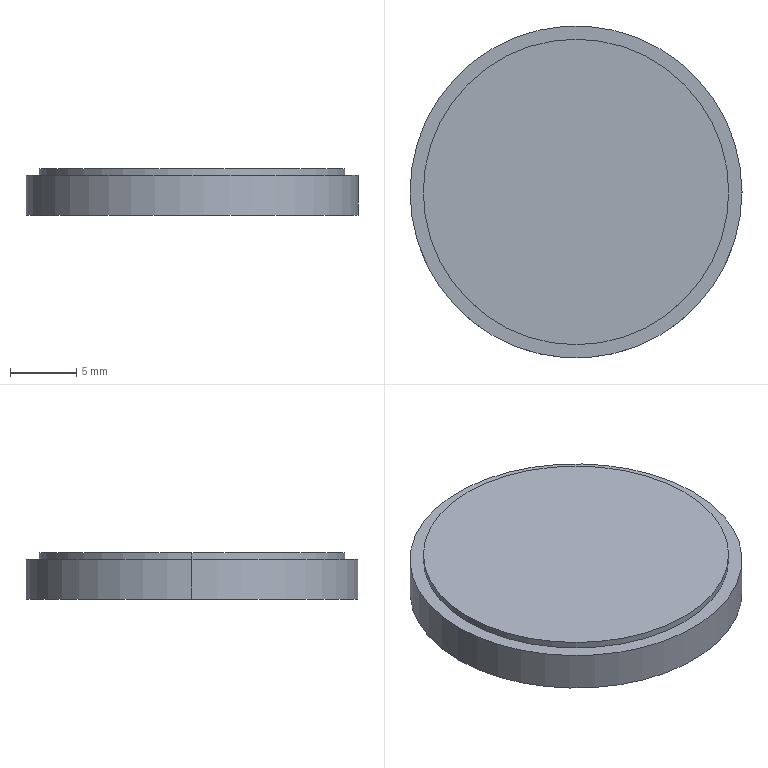Part | STEP file | 7-4-Button1-619-724_Default | 1 solid | 7 faces | box 25 x 25 x 3.5 mm | volume 1680 mm3 | cylinder 4 | plane 3 | commonest cylinder face diameters 23 x2 25 x2
STEP:
#1=CARTESIAN_POINT('',(0.,0.,0.));
#2=DIRECTION('',(0.,0.,1.));
#3=DIRECTION('',(1.,0.,0.));
#4=AXIS2_PLACEMENT_3D('',#1,#2,#3);
#5=CARTESIAN_POINT('',(11.5,0.,0.5));
#6=VERTEX_POINT('',#5);
#7=CARTESIAN_POINT('',(-11.5,0.,0.5));
#8=VERTEX_POINT('',#7);
#9=CARTESIAN_POINT('',(0.,0.,0.5));
#10=DIRECTION('',(0.,0.,1.));
#11=DIRECTION('',(1.,0.,0.));
#12=AXIS2_PLACEMENT_3D('',#9,#10,#11);
#13=CIRCLE('',#12,11.5);
#14=CARTESIAN_POINT('',(0.,0.,0.5));
#15=DIRECTION('',(0.,0.,-1.));
#16=DIRECTION('',(-1.,0.,0.));
#17=AXIS2_PLACEMENT_3D('',#14,#15,#16);
#18=CYLINDRICAL_SURFACE('',#17,11.5);
#19=CARTESIAN_POINT('',(3.142,0.));
#20=DIRECTION('',(-1.,0.));
#21=VECTOR('',#20,1.);
#22=LINE('',#19,#21);
#23=(GEOMETRIC_REPRESENTATION_CONTEXT(2)PARAMETRIC_REPRESENTATION_CONTEXT()REPRESENTATION_CONTEXT('',''));
#24=DEFINITIONAL_REPRESENTATION('',(#22),#23);
#25=PCURVE('',#18,#24);
#26=CARTESIAN_POINT('',(0.,0.,0.5));
#27=DIRECTION('',(0.,0.,1.));
#28=DIRECTION('',(1.,0.,0.));
#29=AXIS2_PLACEMENT_3D('',#26,#27,#28);
#30=PLANE('',#29);
#31=CARTESIAN_POINT('',(0.,0.));
#32=DIRECTION('',(1.,0.));
#33=AXIS2_PLACEMENT_2D('',#31,#32);
#34=CIRCLE('',#33,11.5);
#35=(GEOMETRIC_REPRESENTATION_CONTEXT(2)PARAMETRIC_REPRESENTATION_CONTEXT()REPRESENTATION_CONTEXT('',''));
#36=DEFINITIONAL_REPRESENTATION('',(#34),#35);
#37=PCURVE('',#30,#36);
#38=SURFACE_CURVE('',#13,(#25,#37),.PCURVE_S1.);
#39=EDGE_CURVE('',#6,#8,#38,.T.);
#40=ORIENTED_EDGE('',*,*,#39,.F.);
#41=CARTESIAN_POINT('',(11.5,0.,0.));
#42=VERTEX_POINT('',#41);
#43=CARTESIAN_POINT('',(11.5,0.,0.5));
#44=DIRECTION('',(0.,0.,-1.));
#45=VECTOR('',#44,1.);
#46=LINE('',#43,#45);
#47=CARTESIAN_POINT('',(3.142,0.));
#48=DIRECTION('',(0.,1.));
#49=VECTOR('',#48,1.);
#50=LINE('',#47,#49);
#51=(GEOMETRIC_REPRESENTATION_CONTEXT(2)PARAMETRIC_REPRESENTATION_CONTEXT()REPRESENTATION_CONTEXT('',''));
#52=DEFINITIONAL_REPRESENTATION('',(#50),#51);
#53=PCURVE('',#18,#52);
#54=CARTESIAN_POINT('',(0.,0.,0.5));
#55=DIRECTION('',(0.,0.,-1.));
#56=DIRECTION('',(-1.,0.,0.));
#57=AXIS2_PLACEMENT_3D('',#54,#55,#56);
#58=CYLINDRICAL_SURFACE('',#57,11.5);
#59=CARTESIAN_POINT('',(3.142,0.));
#60=DIRECTION('',(0.,1.));
#61=VECTOR('',#60,1.);
#62=LINE('',#59,#61);
#63=(GEOMETRIC_REPRESENTATION_CONTEXT(2)PARAMETRIC_REPRESENTATION_CONTEXT()REPRESENTATION_CONTEXT('',''));
#64=DEFINITIONAL_REPRESENTATION('',(#62),#63);
#65=PCURVE('',#58,#64);
#66=SURFACE_CURVE('',#46,(#53,#65),.PCURVE_S1.);
#67=EDGE_CURVE('',#6,#42,#66,.T.);
#68=ORIENTED_EDGE('',*,*,#67,.T.);
#69=CARTESIAN_POINT('',(-11.5,0.,0.));
#70=VERTEX_POINT('',#69);
#71=CARTESIAN_POINT('',(0.,0.,0.));
#72=DIRECTION('',(0.,0.,1.));
#73=DIRECTION('',(1.,0.,0.));
#74=AXIS2_PLACEMENT_3D('',#71,#72,#73);
#75=CIRCLE('',#74,11.5);
#76=CARTESIAN_POINT('',(3.142,0.5));
#77=DIRECTION('',(-1.,0.));
#78=VECTOR('',#77,1.);
#79=LINE('',#76,#78);
#80=(GEOMETRIC_REPRESENTATION_CONTEXT(2)PARAMETRIC_REPRESENTATION_CONTEXT()REPRESENTATION_CONTEXT('',''));
#81=DEFINITIONAL_REPRESENTATION('',(#79),#80);
#82=PCURVE('',#18,#81);
#83=CARTESIAN_POINT('',(0.,0.,0.));
#84=DIRECTION('',(0.,0.,1.));
#85=DIRECTION('',(1.,0.,0.));
#86=AXIS2_PLACEMENT_3D('',#83,#84,#85);
#87=PLANE('',#86);
#88=CARTESIAN_POINT('',(0.,0.));
#89=DIRECTION('',(1.,0.));
#90=AXIS2_PLACEMENT_2D('',#88,#89);
#91=CIRCLE('',#90,11.5);
#92=(GEOMETRIC_REPRESENTATION_CONTEXT(2)PARAMETRIC_REPRESENTATION_CONTEXT()REPRESENTATION_CONTEXT('',''));
#93=DEFINITIONAL_REPRESENTATION('',(#91),#92);
#94=PCURVE('',#87,#93);
#95=SURFACE_CURVE('',#75,(#82,#94),.PCURVE_S1.);
#96=EDGE_CURVE('',#42,#70,#95,.T.);
#97=ORIENTED_EDGE('',*,*,#96,.T.);
#98=CARTESIAN_POINT('',(-11.5,0.,0.5));
#99=DIRECTION('',(0.,0.,-1.));
#100=VECTOR('',#99,1.);
#101=LINE('',#98,#100);
#102=CARTESIAN_POINT('',(0.,0.));
#103=DIRECTION('',(0.,1.));
#104=VECTOR('',#103,1.);
#105=LINE('',#102,#104);
#106=(GEOMETRIC_REPRESENTATION_CONTEXT(2)PARAMETRIC_REPRESENTATION_CONTEXT()REPRESENTATION_CONTEXT('',''));
#107=DEFINITIONAL_REPRESENTATION('',(#105),#106);
#108=PCURVE('',#18,#107);
#109=CARTESIAN_POINT('',(6.283,0.));
#110=DIRECTION('',(0.,1.));
#111=VECTOR('',#110,1.);
#112=LINE('',#109,#111);
#113=(GEOMETRIC_REPRESENTATION_CONTEXT(2)PARAMETRIC_REPRESENTATION_CONTEXT()REPRESENTATION_CONTEXT('',''));
#114=DEFINITIONAL_REPRESENTATION('',(#112),#113);
#115=PCURVE('',#58,#114);
#116=SURFACE_CURVE('',#101,(#108,#115),.PCURVE_S1.);
#117=EDGE_CURVE('',#8,#70,#116,.T.);
#118=ORIENTED_EDGE('',*,*,#117,.F.);
#119=EDGE_LOOP('',(#40,#68,#97,#118));
#120=FACE_BOUND('',#119,.T.);
#121=ADVANCED_FACE('',(#120),#18,.T.);
#122=CARTESIAN_POINT('',(12.5,0.,-3.));
#123=VERTEX_POINT('',#122);
#124=CARTESIAN_POINT('',(-12.5,0.,-3.));
#125=VERTEX_POINT('',#124);
#126=CARTESIAN_POINT('',(0.,0.,-3.));
#127=DIRECTION('',(0.,0.,1.));
#128=DIRECTION('',(1.,0.,0.));
#129=AXIS2_PLACEMENT_3D('',#126,#127,#128);
#130=CIRCLE('',#129,12.5);
#131=CARTESIAN_POINT('',(0.,0.,-3.));
#132=DIRECTION('',(0.,0.,1.));
#133=DIRECTION('',(1.,0.,0.));
#134=AXIS2_PLACEMENT_3D('',#131,#132,#133);
#135=CYLINDRICAL_SURFACE('',#134,12.5);
#136=CARTESIAN_POINT('',(0.,0.));
#137=DIRECTION('',(1.,0.));
#138=VECTOR('',#137,1.);
#139=LINE('',#136,#138);
#140=(GEOMETRIC_REPRESENTATION_CONTEXT(2)PARAMETRIC_REPRESENTATION_CONTEXT()REPRESENTATION_CONTEXT('',''));
#141=DEFINITIONAL_REPRESENTATION('',(#139),#140);
#142=PCURVE('',#135,#141);
#143=CARTESIAN_POINT('',(0.,0.,-3.));
#144=DIRECTION('',(0.,0.,1.));
#145=DIRECTION('',(1.,0.,0.));
#146=AXIS2_PLACEMENT_3D('',#143,#144,#145);
#147=PLANE('',#146);
#148=CARTESIAN_POINT('',(0.,0.));
#149=DIRECTION('',(1.,0.));
#150=AXIS2_PLACEMENT_2D('',#148,#149);
#151=CIRCLE('',#150,12.5);
#152=(GEOMETRIC_REPRESENTATION_CONTEXT(2)PARAMETRIC_REPRESENTATION_CONTEXT()REPRESENTATION_CONTEXT('',''));
#153=DEFINITIONAL_REPRESENTATION('',(#151),#152);
#154=PCURVE('',#147,#153);
#155=SURFACE_CURVE('',#130,(#142,#154),.PCURVE_S1.);
#156=EDGE_CURVE('',#123,#125,#155,.T.);
#157=ORIENTED_EDGE('',*,*,#156,.T.);
#158=CARTESIAN_POINT('',(-12.5,0.,0.));
#159=VERTEX_POINT('',#158);
#160=CARTESIAN_POINT('',(-12.5,0.,-3.));
#161=DIRECTION('',(0.,0.,1.));
#162=VECTOR('',#161,1.);
#163=LINE('',#160,#162);
#164=CARTESIAN_POINT('',(3.142,0.));
#165=DIRECTION('',(0.,1.));
#166=VECTOR('',#165,1.);
#167=LINE('',#164,#166);
#168=(GEOMETRIC_REPRESENTATION_CONTEXT(2)PARAMETRIC_REPRESENTATION_CONTEXT()REPRESENTATION_CONTEXT('',''));
#169=DEFINITIONAL_REPRESENTATION('',(#167),#168);
#170=PCURVE('',#135,#169);
#171=CARTESIAN_POINT('',(0.,0.,-3.));
#172=DIRECTION('',(0.,0.,1.));
#173=DIRECTION('',(1.,0.,0.));
#174=AXIS2_PLACEMENT_3D('',#171,#172,#173);
#175=CYLINDRICAL_SURFACE('',#174,12.5);
#176=CARTESIAN_POINT('',(3.142,0.));
#177=DIRECTION('',(0.,1.));
#178=VECTOR('',#177,1.);
#179=LINE('',#176,#178);
#180=(GEOMETRIC_REPRESENTATION_CONTEXT(2)PARAMETRIC_REPRESENTATION_CONTEXT()REPRESENTATION_CONTEXT('',''));
#181=DEFINITIONAL_REPRESENTATION('',(#179),#180);
#182=PCURVE('',#175,#181);
#183=SURFACE_CURVE('',#163,(#170,#182),.PCURVE_S1.);
#184=EDGE_CURVE('',#125,#159,#183,.T.);
#185=ORIENTED_EDGE('',*,*,#184,.T.);
#186=CARTESIAN_POINT('',(12.5,0.,0.));
#187=VERTEX_POINT('',#186);
#188=CARTESIAN_POINT('',(0.,0.,0.));
#189=DIRECTION('',(0.,0.,1.));
#190=DIRECTION('',(1.,0.,0.));
#191=AXIS2_PLACEMENT_3D('',#188,#189,#190);
#192=CIRCLE('',#191,12.5);
#193=CARTESIAN_POINT('',(0.,3.));
#194=DIRECTION('',(1.,0.));
#195=VECTOR('',#194,1.);
#196=LINE('',#193,#195);
#197=(GEOMETRIC_REPRESENTATION_CONTEXT(2)PARAMETRIC_REPRESENTATION_CONTEXT()REPRESENTATION_CONTEXT('',''));
#198=DEFINITIONAL_REPRESENTATION('',(#196),#197);
#199=PCURVE('',#135,#198);
#200=CARTESIAN_POINT('',(0.,0.));
#201=DIRECTION('',(1.,0.));
#202=AXIS2_PLACEMENT_2D('',#200,#201);
#203=CIRCLE('',#202,12.5);
#204=(GEOMETRIC_REPRESENTATION_CONTEXT(2)PARAMETRIC_REPRESENTATION_CONTEXT()REPRESENTATION_CONTEXT('',''));
#205=DEFINITIONAL_REPRESENTATION('',(#203),#204);
#206=PCURVE('',#87,#205);
#207=SURFACE_CURVE('',#192,(#199,#206),.PCURVE_S1.);
#208=EDGE_CURVE('',#187,#159,#207,.T.);
#209=ORIENTED_EDGE('',*,*,#208,.F.);
#210=CARTESIAN_POINT('',(12.5,0.,-3.));
#211=DIRECTION('',(0.,0.,1.));
#212=VECTOR('',#211,1.);
#213=LINE('',#210,#212);
#214=CARTESIAN_POINT('',(0.,0.));
#215=DIRECTION('',(0.,1.));
#216=VECTOR('',#215,1.);
#217=LINE('',#214,#216);
#218=(GEOMETRIC_REPRESENTATION_CONTEXT(2)PARAMETRIC_REPRESENTATION_CONTEXT()REPRESENTATION_CONTEXT('',''));
#219=DEFINITIONAL_REPRESENTATION('',(#217),#218);
#220=PCURVE('',#135,#219);
#221=CARTESIAN_POINT('',(6.283,0.));
#222=DIRECTION('',(0.,1.));
#223=VECTOR('',#222,1.);
#224=LINE('',#221,#223);
#225=(GEOMETRIC_REPRESENTATION_CONTEXT(2)PARAMETRIC_REPRESENTATION_CONTEXT()REPRESENTATION_CONTEXT('',''));
#226=DEFINITIONAL_REPRESENTATION('',(#224),#225);
#227=PCURVE('',#175,#226);
#228=SURFACE_CURVE('',#213,(#220,#227),.PCURVE_S1.);
#229=EDGE_CURVE('',#123,#187,#228,.T.);
#230=ORIENTED_EDGE('',*,*,#229,.F.);
#231=EDGE_LOOP('',(#157,#185,#209,#230));
#232=FACE_BOUND('',#231,.T.);
#233=ADVANCED_FACE('',(#232),#135,.T.);
#234=ORIENTED_EDGE('',*,*,#208,.T.);
#235=CARTESIAN_POINT('',(0.,0.,0.));
#236=DIRECTION('',(0.,0.,1.));
#237=DIRECTION('',(1.,0.,0.));
#238=AXIS2_PLACEMENT_3D('',#235,#236,#237);
#239=CIRCLE('',#238,12.5);
#240=CARTESIAN_POINT('',(0.,0.));
#241=DIRECTION('',(1.,0.));
#242=AXIS2_PLACEMENT_2D('',#240,#241);
#243=CIRCLE('',#242,12.5);
#244=(GEOMETRIC_REPRESENTATION_CONTEXT(2)PARAMETRIC_REPRESENTATION_CONTEXT()REPRESENTATION_CONTEXT('',''));
#245=DEFINITIONAL_REPRESENTATION('',(#243),#244);
#246=PCURVE('',#87,#245);
#247=CARTESIAN_POINT('',(0.,3.));
#248=DIRECTION('',(1.,0.));
#249=VECTOR('',#248,1.);
#250=LINE('',#247,#249);
#251=(GEOMETRIC_REPRESENTATION_CONTEXT(2)PARAMETRIC_REPRESENTATION_CONTEXT()REPRESENTATION_CONTEXT('',''));
#252=DEFINITIONAL_REPRESENTATION('',(#250),#251);
#253=PCURVE('',#175,#252);
#254=SURFACE_CURVE('',#239,(#246,#253),.PCURVE_S1.);
#255=EDGE_CURVE('',#159,#187,#254,.T.);
#256=ORIENTED_EDGE('',*,*,#255,.T.);
#257=EDGE_LOOP('',(#234,#256));
#258=FACE_BOUND('',#257,.T.);
#259=CARTESIAN_POINT('',(0.,0.,0.));
#260=DIRECTION('',(0.,0.,1.));
#261=DIRECTION('',(1.,0.,0.));
#262=AXIS2_PLACEMENT_3D('',#259,#260,#261);
#263=CIRCLE('',#262,11.5);
#264=CARTESIAN_POINT('',(0.,0.));
#265=DIRECTION('',(1.,0.));
#266=AXIS2_PLACEMENT_2D('',#264,#265);
#267=CIRCLE('',#266,11.5);
#268=(GEOMETRIC_REPRESENTATION_CONTEXT(2)PARAMETRIC_REPRESENTATION_CONTEXT()REPRESENTATION_CONTEXT('',''));
#269=DEFINITIONAL_REPRESENTATION('',(#267),#268);
#270=PCURVE('',#87,#269);
#271=CARTESIAN_POINT('',(9.425,0.5));
#272=DIRECTION('',(-1.,0.));
#273=VECTOR('',#272,1.);
#274=LINE('',#271,#273);
#275=(GEOMETRIC_REPRESENTATION_CONTEXT(2)PARAMETRIC_REPRESENTATION_CONTEXT()REPRESENTATION_CONTEXT('',''));
#276=DEFINITIONAL_REPRESENTATION('',(#274),#275);
#277=PCURVE('',#58,#276);
#278=SURFACE_CURVE('',#263,(#270,#277),.PCURVE_S1.);
#279=EDGE_CURVE('',#70,#42,#278,.T.);
#280=ORIENTED_EDGE('',*,*,#279,.F.);
#281=ORIENTED_EDGE('',*,*,#96,.F.);
#282=EDGE_LOOP('',(#280,#281));
#283=FACE_BOUND('',#282,.T.);
#284=ADVANCED_FACE('',(#258,#283),#87,.T.);
#285=ORIENTED_EDGE('',*,*,#184,.F.);
#286=CARTESIAN_POINT('',(0.,0.,-3.));
#287=DIRECTION('',(0.,0.,1.));
#288=DIRECTION('',(1.,0.,0.));
#289=AXIS2_PLACEMENT_3D('',#286,#287,#288);
#290=CIRCLE('',#289,12.5);
#291=CARTESIAN_POINT('',(0.,0.));
#292=DIRECTION('',(1.,0.));
#293=VECTOR('',#292,1.);
#294=LINE('',#291,#293);
#295=(GEOMETRIC_REPRESENTATION_CONTEXT(2)PARAMETRIC_REPRESENTATION_CONTEXT()REPRESENTATION_CONTEXT('',''));
#296=DEFINITIONAL_REPRESENTATION('',(#294),#295);
#297=PCURVE('',#175,#296);
#298=CARTESIAN_POINT('',(0.,0.));
#299=DIRECTION('',(1.,0.));
#300=AXIS2_PLACEMENT_2D('',#298,#299);
#301=CIRCLE('',#300,12.5);
#302=(GEOMETRIC_REPRESENTATION_CONTEXT(2)PARAMETRIC_REPRESENTATION_CONTEXT()REPRESENTATION_CONTEXT('',''));
#303=DEFINITIONAL_REPRESENTATION('',(#301),#302);
#304=PCURVE('',#147,#303);
#305=SURFACE_CURVE('',#290,(#297,#304),.PCURVE_S1.);
#306=EDGE_CURVE('',#125,#123,#305,.T.);
#307=ORIENTED_EDGE('',*,*,#306,.T.);
#308=ORIENTED_EDGE('',*,*,#229,.T.);
#309=ORIENTED_EDGE('',*,*,#255,.F.);
#310=EDGE_LOOP('',(#285,#307,#308,#309));
#311=FACE_BOUND('',#310,.T.);
#312=ADVANCED_FACE('',(#311),#175,.T.);
#313=ORIENTED_EDGE('',*,*,#156,.F.);
#314=ORIENTED_EDGE('',*,*,#306,.F.);
#315=EDGE_LOOP('',(#313,#314));
#316=FACE_BOUND('',#315,.T.);
#317=ADVANCED_FACE('',(#316),#147,.F.);
#318=ORIENTED_EDGE('',*,*,#67,.F.);
#319=CARTESIAN_POINT('',(0.,0.,0.5));
#320=DIRECTION('',(0.,0.,1.));
#321=DIRECTION('',(1.,0.,0.));
#322=AXIS2_PLACEMENT_3D('',#319,#320,#321);
#323=CIRCLE('',#322,11.5);
#324=CARTESIAN_POINT('',(9.425,0.));
#325=DIRECTION('',(-1.,0.));
#326=VECTOR('',#325,1.);
#327=LINE('',#324,#326);
#328=(GEOMETRIC_REPRESENTATION_CONTEXT(2)PARAMETRIC_REPRESENTATION_CONTEXT()REPRESENTATION_CONTEXT('',''));
#329=DEFINITIONAL_REPRESENTATION('',(#327),#328);
#330=PCURVE('',#58,#329);
#331=CARTESIAN_POINT('',(0.,0.));
#332=DIRECTION('',(1.,0.));
#333=AXIS2_PLACEMENT_2D('',#331,#332);
#334=CIRCLE('',#333,11.5);
#335=(GEOMETRIC_REPRESENTATION_CONTEXT(2)PARAMETRIC_REPRESENTATION_CONTEXT()REPRESENTATION_CONTEXT('',''));
#336=DEFINITIONAL_REPRESENTATION('',(#334),#335);
#337=PCURVE('',#30,#336);
#338=SURFACE_CURVE('',#323,(#330,#337),.PCURVE_S1.);
#339=EDGE_CURVE('',#8,#6,#338,.T.);
#340=ORIENTED_EDGE('',*,*,#339,.F.);
#341=ORIENTED_EDGE('',*,*,#117,.T.);
#342=ORIENTED_EDGE('',*,*,#279,.T.);
#343=EDGE_LOOP('',(#318,#340,#341,#342));
#344=FACE_BOUND('',#343,.T.);
#345=ADVANCED_FACE('',(#344),#58,.T.);
#346=ORIENTED_EDGE('',*,*,#339,.T.);
#347=ORIENTED_EDGE('',*,*,#39,.T.);
#348=EDGE_LOOP('',(#346,#347));
#349=FACE_BOUND('',#348,.T.);
#350=ADVANCED_FACE('',(#349),#30,.T.);
#351=CLOSED_SHELL('',(#121,#233,#284,#312,#317,#345,#350));
#352=MANIFOLD_SOLID_BREP('',#351);
#353=(LENGTH_UNIT()NAMED_UNIT(*)SI_UNIT(.MILLI.,.METRE.));
#354=UNCERTAINTY_MEASURE_WITH_UNIT(LENGTH_MEASURE(0.0000001),#353,'','');
#355=(NAMED_UNIT(*)PLANE_ANGLE_UNIT()SI_UNIT($,.RADIAN.));
#356=(NAMED_UNIT(*)SI_UNIT($,.STERADIAN.)SOLID_ANGLE_UNIT());
#357=(GEOMETRIC_REPRESENTATION_CONTEXT(3)GLOBAL_UNCERTAINTY_ASSIGNED_CONTEXT((#354))GLOBAL_UNIT_ASSIGNED_CONTEXT((#353,#355,#356))REPRESENTATION_CONTEXT('',''));
#358=ADVANCED_BREP_SHAPE_REPRESENTATION('',(#4,#352),#357);